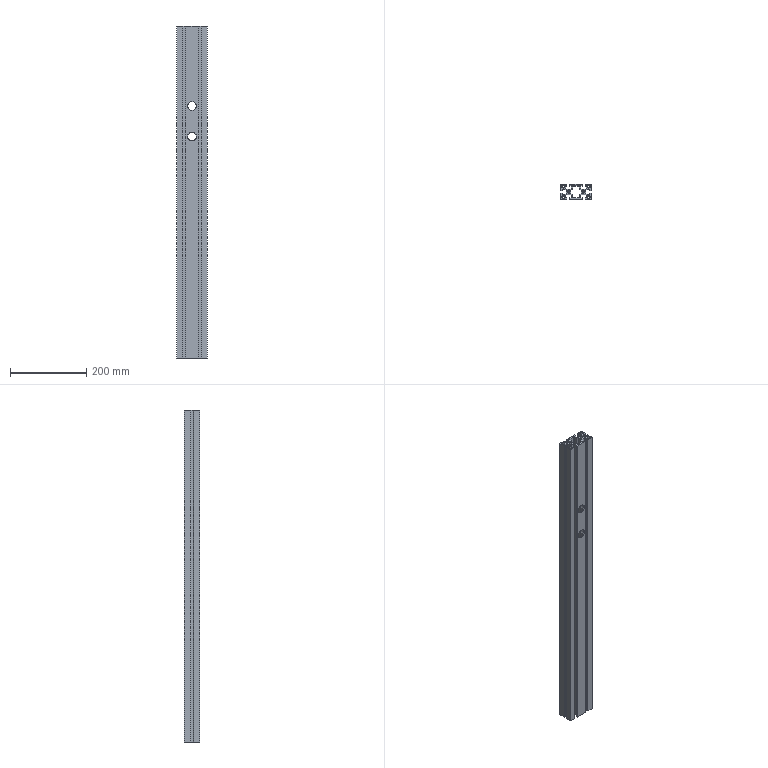Part | NX | 1 solid | 112 faces | box 80 x 40 x 871 mm | volume 1047449 mm3 | plane 90 | cylinder 22 | commonest cylinder face diameters 6 x12 8 x4 23 x4 6.75 x2